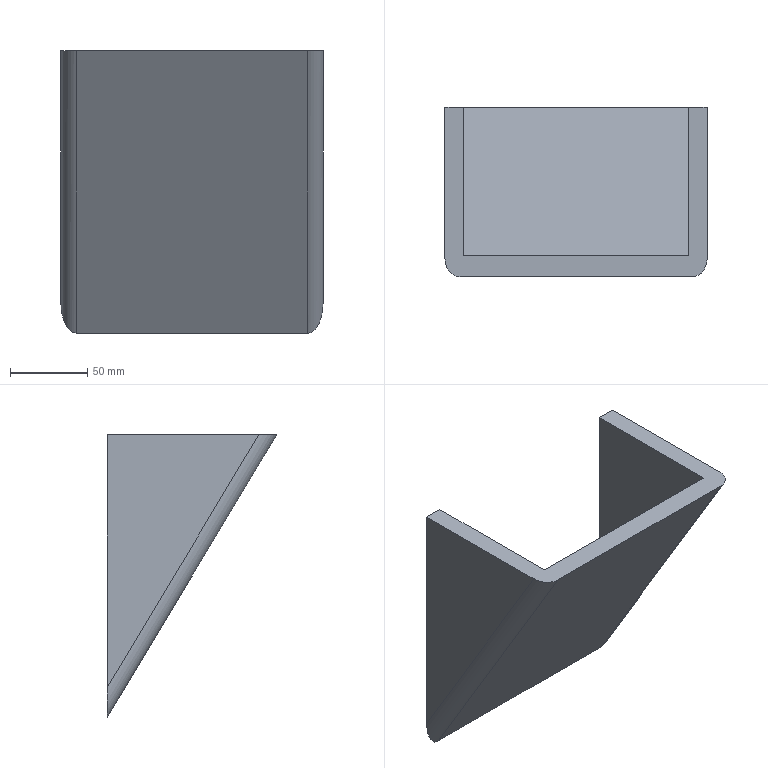Part | SolidWorks | features Extrusion 1, Fillet 1, ICE 1, Shell 1 | 1 solid | 10 faces | box 170 x 110 x 183 mm | volume 582886 mm3 | plane 8 | cylinder 2 | commonest cylinder face diameters 20 x2
STEP:
#1=CARTESIAN_POINT('',(73.,55.,386.948));
#2=VERTEX_POINT('',#1);
#3=CARTESIAN_POINT('',(73.,55.,227.241));
#4=VERTEX_POINT('',#3);
#5=CARTESIAN_POINT('',(73.,55.,500.));
#6=DIRECTION('',(0.,0.,-1.));
#7=VECTOR('',#6,1000.);
#8=LINE('',#5,#7);
#9=EDGE_CURVE('',#2,#4,#8,.T.);
#10=ORIENTED_EDGE('',*,*,#9,.F.);
#11=CARTESIAN_POINT('',(85.,55.,386.948));
#12=VERTEX_POINT('',#11);
#13=CARTESIAN_POINT('',(115.,55.,386.948));
#14=DIRECTION('',(-1.,0.,0.));
#15=VECTOR('',#14,1000.);
#16=LINE('',#13,#15);
#17=EDGE_CURVE('',#12,#2,#16,.T.);
#18=ORIENTED_EDGE('',*,*,#17,.F.);
#19=CARTESIAN_POINT('',(85.,55.,223.359));
#20=VERTEX_POINT('',#19);
#21=CARTESIAN_POINT('',(85.,55.,500.));
#22=DIRECTION('',(0.,0.,-1.));
#23=VECTOR('',#22,1000.);
#24=LINE('',#21,#23);
#25=EDGE_CURVE('',#12,#20,#24,.T.);
#26=ORIENTED_EDGE('',*,*,#25,.T.);
#27=CARTESIAN_POINT('',(75.,55.,203.948));
#28=VERTEX_POINT('',#27);
#29=CARTESIAN_POINT('',(85.,55.,223.359));
#30=CARTESIAN_POINT('',(85.,55.,211.988));
#31=CARTESIAN_POINT('',(80.858,55.,203.948));
#32=CARTESIAN_POINT('',(75.,55.,203.948));
#33=(BOUNDED_CURVE()B_SPLINE_CURVE(3,(#29,#30,#31,#32),.UNSPECIFIED.,.F.,.F.)B_SPLINE_CURVE_WITH_KNOTS((4,4),(4.712,6.283),.UNSPECIFIED.)CURVE()GEOMETRIC_REPRESENTATION_ITEM()RATIONAL_B_SPLINE_CURVE((1.,0.8047,0.8047,1.))REPRESENTATION_ITEM(''));
#34=EDGE_CURVE('',#20,#28,#33,.T.);
#35=ORIENTED_EDGE('',*,*,#34,.T.);
#36=CARTESIAN_POINT('',(-75.,55.,203.948));
#37=VERTEX_POINT('',#36);
#38=CARTESIAN_POINT('',(115.,55.,203.948));
#39=DIRECTION('',(-1.,0.,0.));
#40=VECTOR('',#39,1000.);
#41=LINE('',#38,#40);
#42=EDGE_CURVE('',#28,#37,#41,.T.);
#43=ORIENTED_EDGE('',*,*,#42,.T.);
#44=CARTESIAN_POINT('',(-85.,55.,223.359));
#45=VERTEX_POINT('',#44);
#46=CARTESIAN_POINT('',(-75.,55.,203.948));
#47=CARTESIAN_POINT('',(-80.858,55.,203.948));
#48=CARTESIAN_POINT('',(-85.,55.,211.988));
#49=CARTESIAN_POINT('',(-85.,55.,223.359));
#50=(BOUNDED_CURVE()B_SPLINE_CURVE(3,(#46,#47,#48,#49),.UNSPECIFIED.,.F.,.F.)B_SPLINE_CURVE_WITH_KNOTS((4,4),(0.,1.571),.UNSPECIFIED.)CURVE()GEOMETRIC_REPRESENTATION_ITEM()RATIONAL_B_SPLINE_CURVE((1.,0.8047,0.8047,1.))REPRESENTATION_ITEM(''));
#51=EDGE_CURVE('',#37,#45,#50,.T.);
#52=ORIENTED_EDGE('',*,*,#51,.T.);
#53=CARTESIAN_POINT('',(-85.,55.,386.948));
#54=VERTEX_POINT('',#53);
#55=CARTESIAN_POINT('',(-85.,55.,500.));
#56=DIRECTION('',(0.,0.,-1.));
#57=VECTOR('',#56,1000.);
#58=LINE('',#55,#57);
#59=EDGE_CURVE('',#54,#45,#58,.T.);
#60=ORIENTED_EDGE('',*,*,#59,.F.);
#61=CARTESIAN_POINT('',(-73.,55.,386.948));
#62=VERTEX_POINT('',#61);
#63=CARTESIAN_POINT('',(115.,55.,386.948));
#64=DIRECTION('',(-1.,0.,0.));
#65=VECTOR('',#64,1000.);
#66=LINE('',#63,#65);
#67=EDGE_CURVE('',#62,#54,#66,.T.);
#68=ORIENTED_EDGE('',*,*,#67,.F.);
#69=CARTESIAN_POINT('',(-73.,55.,227.241));
#70=VERTEX_POINT('',#69);
#71=CARTESIAN_POINT('',(-73.,55.,500.));
#72=DIRECTION('',(0.,0.,-1.));
#73=VECTOR('',#72,1000.);
#74=LINE('',#71,#73);
#75=EDGE_CURVE('',#62,#70,#74,.T.);
#76=ORIENTED_EDGE('',*,*,#75,.T.);
#77=CARTESIAN_POINT('',(115.,55.,227.241));
#78=DIRECTION('',(-1.,0.,0.));
#79=VECTOR('',#78,1000.);
#80=LINE('',#77,#79);
#81=EDGE_CURVE('',#4,#70,#80,.T.);
#82=ORIENTED_EDGE('',*,*,#81,.F.);
#83=EDGE_LOOP('',(#10,#18,#26,#35,#43,#52,#60,#68,#76,#82));
#84=FACE_OUTER_BOUND('',#83,.T.);
#85=CARTESIAN_POINT('',(85.,55.,500.));
#86=DIRECTION('',(0.,-1.,0.));
#87=DIRECTION('',(1.,0.,0.));
#88=AXIS2_PLACEMENT_3D('',#85,#86,#87);
#89=PLANE('',#88);
#90=ADVANCED_FACE('',(#84),#89,.F.);
#91=ORIENTED_EDGE('',*,*,#17,.T.);
#92=CARTESIAN_POINT('',(73.,-40.999,386.948));
#93=VERTEX_POINT('',#92);
#94=CARTESIAN_POINT('',(73.,55.,386.948));
#95=DIRECTION('',(0.,-1.,0.));
#96=VECTOR('',#95,1000.);
#97=LINE('',#94,#96);
#98=EDGE_CURVE('',#2,#93,#97,.T.);
#99=ORIENTED_EDGE('',*,*,#98,.T.);
#100=CARTESIAN_POINT('',(-73.,-40.999,386.948));
#101=VERTEX_POINT('',#100);
#102=CARTESIAN_POINT('',(115.,-40.999,386.948));
#103=DIRECTION('',(-1.,0.,0.));
#104=VECTOR('',#103,1000.);
#105=LINE('',#102,#104);
#106=EDGE_CURVE('',#93,#101,#105,.T.);
#107=ORIENTED_EDGE('',*,*,#106,.T.);
#108=CARTESIAN_POINT('',(-73.,55.,386.948));
#109=DIRECTION('',(0.,1.,0.));
#110=VECTOR('',#109,1000.);
#111=LINE('',#108,#110);
#112=EDGE_CURVE('',#101,#62,#111,.T.);
#113=ORIENTED_EDGE('',*,*,#112,.T.);
#114=ORIENTED_EDGE('',*,*,#67,.T.);
#115=CARTESIAN_POINT('',(-85.,-43.332,386.948));
#116=VERTEX_POINT('',#115);
#117=CARTESIAN_POINT('',(-85.,55.,386.948));
#118=DIRECTION('',(0.,1.,0.));
#119=VECTOR('',#118,1000.);
#120=LINE('',#117,#119);
#121=EDGE_CURVE('',#116,#54,#120,.T.);
#122=ORIENTED_EDGE('',*,*,#121,.F.);
#123=CARTESIAN_POINT('',(-75.,-55.,386.948));
#124=VERTEX_POINT('',#123);
#125=CARTESIAN_POINT('',(-85.,-43.332,386.948));
#126=CARTESIAN_POINT('',(-85.,-50.167,386.948));
#127=CARTESIAN_POINT('',(-80.858,-55.,386.948));
#128=CARTESIAN_POINT('',(-75.,-55.,386.948));
#129=(BOUNDED_CURVE()B_SPLINE_CURVE(3,(#125,#126,#127,#128),.UNSPECIFIED.,.F.,.F.)B_SPLINE_CURVE_WITH_KNOTS((4,4),(1.571,3.142),.UNSPECIFIED.)CURVE()GEOMETRIC_REPRESENTATION_ITEM()RATIONAL_B_SPLINE_CURVE((1.,0.8047,0.8047,1.))REPRESENTATION_ITEM(''));
#130=EDGE_CURVE('',#116,#124,#129,.T.);
#131=ORIENTED_EDGE('',*,*,#130,.T.);
#132=CARTESIAN_POINT('',(75.,-55.,386.948));
#133=VERTEX_POINT('',#132);
#134=CARTESIAN_POINT('',(115.,-55.,386.948));
#135=DIRECTION('',(-1.,0.,0.));
#136=VECTOR('',#135,1000.);
#137=LINE('',#134,#136);
#138=EDGE_CURVE('',#133,#124,#137,.T.);
#139=ORIENTED_EDGE('',*,*,#138,.F.);
#140=CARTESIAN_POINT('',(85.,-43.332,386.948));
#141=VERTEX_POINT('',#140);
#142=CARTESIAN_POINT('',(75.,-55.,386.948));
#143=CARTESIAN_POINT('',(80.858,-55.,386.948));
#144=CARTESIAN_POINT('',(85.,-50.167,386.948));
#145=CARTESIAN_POINT('',(85.,-43.332,386.948));
#146=(BOUNDED_CURVE()B_SPLINE_CURVE(3,(#142,#143,#144,#145),.UNSPECIFIED.,.F.,.T.)B_SPLINE_CURVE_WITH_KNOTS((4,4),(3.142,4.712),.UNSPECIFIED.)CURVE()GEOMETRIC_REPRESENTATION_ITEM()RATIONAL_B_SPLINE_CURVE((1.,0.8047,0.8047,1.))REPRESENTATION_ITEM(''));
#147=EDGE_CURVE('',#133,#141,#146,.T.);
#148=ORIENTED_EDGE('',*,*,#147,.T.);
#149=CARTESIAN_POINT('',(85.,55.,386.948));
#150=DIRECTION('',(0.,-1.,0.));
#151=VECTOR('',#150,1000.);
#152=LINE('',#149,#151);
#153=EDGE_CURVE('',#12,#141,#152,.T.);
#154=ORIENTED_EDGE('',*,*,#153,.F.);
#155=EDGE_LOOP('',(#91,#99,#107,#113,#114,#122,#131,#139,#148,#154));
#156=FACE_OUTER_BOUND('',#155,.T.);
#157=CARTESIAN_POINT('',(115.,55.,386.948));
#158=DIRECTION('',(0.,0.,1.));
#159=DIRECTION('',(1.,0.,0.));
#160=AXIS2_PLACEMENT_3D('',#157,#158,#159);
#161=PLANE('',#160);
#162=ADVANCED_FACE('',(#156),#161,.T.);
#163=ORIENTED_EDGE('',*,*,#153,.T.);
#164=CARTESIAN_POINT('',(85.,-67.152,426.575));
#165=DIRECTION('',(0.,0.5152,-0.8571));
#166=VECTOR('',#165,1000.);
#167=LINE('',#164,#166);
#168=EDGE_CURVE('',#141,#20,#167,.T.);
#169=ORIENTED_EDGE('',*,*,#168,.T.);
#170=ORIENTED_EDGE('',*,*,#25,.F.);
#171=EDGE_LOOP('',(#163,#169,#170));
#172=FACE_OUTER_BOUND('',#171,.T.);
#173=CARTESIAN_POINT('',(85.,55.,500.));
#174=DIRECTION('',(1.,0.,0.));
#175=DIRECTION('',(0.,0.,-1.));
#176=AXIS2_PLACEMENT_3D('',#173,#174,#175);
#177=PLANE('',#176);
#178=ADVANCED_FACE('',(#172),#177,.T.);
#179=ORIENTED_EDGE('',*,*,#59,.T.);
#180=CARTESIAN_POINT('',(-85.,-46.429,392.1));
#181=DIRECTION('',(0.,-0.5152,0.8571));
#182=VECTOR('',#181,1000.);
#183=LINE('',#180,#182);
#184=EDGE_CURVE('',#45,#116,#183,.T.);
#185=ORIENTED_EDGE('',*,*,#184,.T.);
#186=ORIENTED_EDGE('',*,*,#121,.T.);
#187=EDGE_LOOP('',(#179,#185,#186));
#188=FACE_OUTER_BOUND('',#187,.T.);
#189=CARTESIAN_POINT('',(-85.,55.,500.));
#190=DIRECTION('',(1.,0.,0.));
#191=DIRECTION('',(0.,1.,0.));
#192=AXIS2_PLACEMENT_3D('',#189,#190,#191);
#193=PLANE('',#192);
#194=ADVANCED_FACE('',(#188),#193,.F.);
#195=ORIENTED_EDGE('',*,*,#42,.F.);
#196=CARTESIAN_POINT('',(75.,-55.,386.948));
#197=DIRECTION('',(0.,-0.5152,0.8571));
#198=VECTOR('',#197,1000.);
#199=LINE('',#196,#198);
#200=EDGE_CURVE('',#28,#133,#199,.T.);
#201=ORIENTED_EDGE('',*,*,#200,.T.);
#202=ORIENTED_EDGE('',*,*,#138,.T.);
#203=CARTESIAN_POINT('',(-75.,55.,203.948));
#204=DIRECTION('',(0.,0.5152,-0.8571));
#205=VECTOR('',#204,1000.);
#206=LINE('',#203,#205);
#207=EDGE_CURVE('',#124,#37,#206,.T.);
#208=ORIENTED_EDGE('',*,*,#207,.T.);
#209=EDGE_LOOP('',(#195,#201,#202,#208));
#210=FACE_OUTER_BOUND('',#209,.T.);
#211=CARTESIAN_POINT('',(115.,-55.,386.948));
#212=DIRECTION('',(0.,-0.8571,-0.5152));
#213=DIRECTION('',(0.,0.5152,-0.8571));
#214=AXIS2_PLACEMENT_3D('',#211,#212,#213);
#215=PLANE('',#214);
#216=ADVANCED_FACE('',(#210),#215,.T.);
#217=ORIENTED_EDGE('',*,*,#147,.F.);
#218=ORIENTED_EDGE('',*,*,#200,.F.);
#219=ORIENTED_EDGE('',*,*,#34,.F.);
#220=ORIENTED_EDGE('',*,*,#168,.F.);
#221=EDGE_LOOP('',(#217,#218,#219,#220));
#222=FACE_OUTER_BOUND('',#221,.T.);
#223=CARTESIAN_POINT('',(75.,-67.152,426.575));
#224=DIRECTION('',(0.,0.5152,-0.8571));
#225=DIRECTION('',(0.,0.8571,0.5152));
#226=AXIS2_PLACEMENT_3D('',#223,#224,#225);
#227=CYLINDRICAL_SURFACE('',#226,10.);
#228=ADVANCED_FACE('',(#222),#227,.T.);
#229=ORIENTED_EDGE('',*,*,#51,.F.);
#230=ORIENTED_EDGE('',*,*,#207,.F.);
#231=ORIENTED_EDGE('',*,*,#130,.F.);
#232=ORIENTED_EDGE('',*,*,#184,.F.);
#233=EDGE_LOOP('',(#229,#230,#231,#232));
#234=FACE_OUTER_BOUND('',#233,.T.);
#235=CARTESIAN_POINT('',(-75.,-67.152,426.575));
#236=DIRECTION('',(0.,0.5152,-0.8571));
#237=DIRECTION('',(0.,0.8571,0.5152));
#238=AXIS2_PLACEMENT_3D('',#235,#236,#237);
#239=CYLINDRICAL_SURFACE('',#238,10.);
#240=ADVANCED_FACE('',(#234),#239,.T.);
#241=ORIENTED_EDGE('',*,*,#98,.F.);
#242=ORIENTED_EDGE('',*,*,#9,.T.);
#243=CARTESIAN_POINT('',(73.,-44.715,393.131));
#244=DIRECTION('',(0.,-0.5152,0.8571));
#245=VECTOR('',#244,1000.);
#246=LINE('',#243,#245);
#247=EDGE_CURVE('',#4,#93,#246,.T.);
#248=ORIENTED_EDGE('',*,*,#247,.T.);
#249=EDGE_LOOP('',(#241,#242,#248));
#250=FACE_OUTER_BOUND('',#249,.T.);
#251=CARTESIAN_POINT('',(73.,55.,500.));
#252=DIRECTION('',(1.,0.,0.));
#253=DIRECTION('',(0.,0.,-1.));
#254=AXIS2_PLACEMENT_3D('',#251,#252,#253);
#255=PLANE('',#254);
#256=ADVANCED_FACE('',(#250),#255,.F.);
#257=ORIENTED_EDGE('',*,*,#75,.F.);
#258=ORIENTED_EDGE('',*,*,#112,.F.);
#259=CARTESIAN_POINT('',(-73.,-65.438,427.606));
#260=DIRECTION('',(0.,0.5152,-0.8571));
#261=VECTOR('',#260,1000.);
#262=LINE('',#259,#261);
#263=EDGE_CURVE('',#101,#70,#262,.T.);
#264=ORIENTED_EDGE('',*,*,#263,.T.);
#265=EDGE_LOOP('',(#257,#258,#264));
#266=FACE_OUTER_BOUND('',#265,.T.);
#267=CARTESIAN_POINT('',(-73.,55.,500.));
#268=DIRECTION('',(1.,0.,0.));
#269=DIRECTION('',(0.,1.,0.));
#270=AXIS2_PLACEMENT_3D('',#267,#268,#269);
#271=PLANE('',#270);
#272=ADVANCED_FACE('',(#266),#271,.T.);
#273=ORIENTED_EDGE('',*,*,#81,.T.);
#274=ORIENTED_EDGE('',*,*,#263,.F.);
#275=ORIENTED_EDGE('',*,*,#106,.F.);
#276=ORIENTED_EDGE('',*,*,#247,.F.);
#277=EDGE_LOOP('',(#273,#274,#275,#276));
#278=FACE_OUTER_BOUND('',#277,.T.);
#279=CARTESIAN_POINT('',(115.,-44.715,393.131));
#280=DIRECTION('',(0.,-0.8571,-0.5152));
#281=DIRECTION('',(0.,0.5152,-0.8571));
#282=AXIS2_PLACEMENT_3D('',#279,#280,#281);
#283=PLANE('',#282);
#284=ADVANCED_FACE('',(#278),#283,.F.);
#285=CLOSED_SHELL('',(#90,#162,#178,#194,#216,#228,#240,#256,#272,#284));
#286=MANIFOLD_SOLID_BREP('',#285);
#287=CARTESIAN_POINT('',(0.,0.,0.));
#288=DIRECTION('',(0.,0.,1.));
#289=DIRECTION('',(1.,0.,0.));
#290=AXIS2_PLACEMENT_3D('',#287,#288,#289);
#291=(LENGTH_UNIT()NAMED_UNIT(*)SI_UNIT(.MILLI.,.METRE.));
#292=UNCERTAINTY_MEASURE_WITH_UNIT(LENGTH_MEASURE(0.00001),#291,'','');
#293=(NAMED_UNIT(*)PLANE_ANGLE_UNIT()SI_UNIT($,.RADIAN.));
#294=(NAMED_UNIT(*)SI_UNIT($,.STERADIAN.)SOLID_ANGLE_UNIT());
#295=(GEOMETRIC_REPRESENTATION_CONTEXT(3)GLOBAL_UNCERTAINTY_ASSIGNED_CONTEXT((#292))GLOBAL_UNIT_ASSIGNED_CONTEXT((#291,#293,#294))REPRESENTATION_CONTEXT('',''));
#296=ADVANCED_BREP_SHAPE_REPRESENTATION('',(#286,#290),#295);